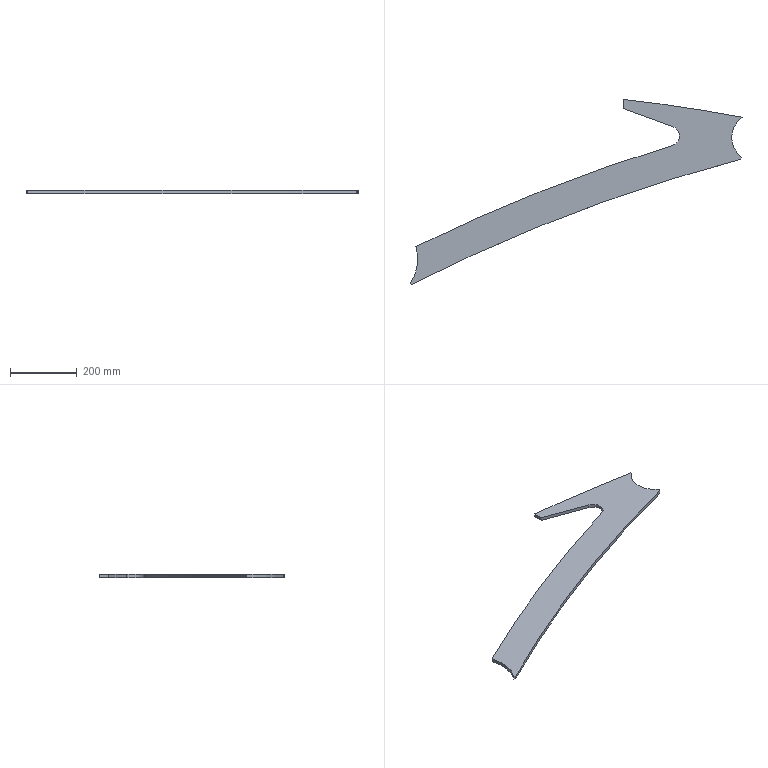Part | SolidWorks | features Extrusion 1 | 1 solid | 14 faces | box 997.777 x 556.587 x 10 mm | volume 1190658 mm3 | cylinder 7 | plane 7 | commonest cylinder face diameters 146 x2 60 x1 256 x1 9968 x1 10024 x1 10216 x1
STEP:
#1=CARTESIAN_POINT('',(1102.629,425.298,10.));
#2=VERTEX_POINT('',#1);
#3=CARTESIAN_POINT('',(1071.5,365.5,10.));
#4=VERTEX_POINT('',#3);
#5=CARTESIAN_POINT('',(1144.5,365.5,10.));
#6=DIRECTION('',(0.,0.,1.));
#7=DIRECTION('',(1.,0.,0.));
#8=AXIS2_PLACEMENT_3D('',#5,#6,#7);
#9=CIRCLE('',#8,73.);
#10=EDGE_CURVE('',#2,#4,#9,.T.);
#11=ORIENTED_EDGE('',*,*,#10,.T.);
#12=CARTESIAN_POINT('',(1071.5,365.5,0.));
#13=VERTEX_POINT('',#12);
#14=CARTESIAN_POINT('',(1071.5,365.5,10.));
#15=DIRECTION('',(0.,0.,-1.));
#16=VECTOR('',#15,1000.);
#17=LINE('',#14,#16);
#18=EDGE_CURVE('',#4,#13,#17,.T.);
#19=ORIENTED_EDGE('',*,*,#18,.T.);
#20=CARTESIAN_POINT('',(1102.629,425.298,0.));
#21=VERTEX_POINT('',#20);
#22=CARTESIAN_POINT('',(1144.5,365.5,0.));
#23=DIRECTION('',(0.,0.,1.));
#24=DIRECTION('',(1.,0.,0.));
#25=AXIS2_PLACEMENT_3D('',#22,#23,#24);
#26=CIRCLE('',#25,73.);
#27=EDGE_CURVE('',#21,#13,#26,.T.);
#28=ORIENTED_EDGE('',*,*,#27,.F.);
#29=CARTESIAN_POINT('',(1102.629,425.298,10.));
#30=DIRECTION('',(0.,0.,-1.));
#31=VECTOR('',#30,1000.);
#32=LINE('',#29,#31);
#33=EDGE_CURVE('',#2,#21,#32,.T.);
#34=ORIENTED_EDGE('',*,*,#33,.F.);
#35=EDGE_LOOP('',(#11,#19,#28,#34));
#36=FACE_OUTER_BOUND('',#35,.T.);
#37=CARTESIAN_POINT('',(1144.5,365.5,10.));
#38=DIRECTION('',(0.,0.,-1.));
#39=DIRECTION('',(-1.,0.,0.));
#40=AXIS2_PLACEMENT_3D('',#37,#38,#39);
#41=CYLINDRICAL_SURFACE('',#40,73.);
#42=ADVANCED_FACE('',(#36),#41,.F.);
#43=CARTESIAN_POINT('',(893.221,341.536,0.));
#44=VERTEX_POINT('',#43);
#45=CARTESIAN_POINT('',(894.771,398.434,0.));
#46=VERTEX_POINT('',#45);
#47=CARTESIAN_POINT('',(884.51,370.243,0.));
#48=DIRECTION('',(0.,0.,1.));
#49=DIRECTION('',(1.,0.,0.));
#50=AXIS2_PLACEMENT_3D('',#47,#48,#49);
#51=CIRCLE('',#50,30.);
#52=EDGE_CURVE('',#44,#46,#51,.T.);
#53=ORIENTED_EDGE('',*,*,#52,.F.);
#54=CARTESIAN_POINT('',(893.221,341.536,10.));
#55=VERTEX_POINT('',#54);
#56=CARTESIAN_POINT('',(893.221,341.536,10.));
#57=DIRECTION('',(0.,0.,-1.));
#58=VECTOR('',#57,1000.);
#59=LINE('',#56,#58);
#60=EDGE_CURVE('',#55,#44,#59,.T.);
#61=ORIENTED_EDGE('',*,*,#60,.F.);
#62=CARTESIAN_POINT('',(894.771,398.434,10.));
#63=VERTEX_POINT('',#62);
#64=CARTESIAN_POINT('',(884.51,370.243,10.));
#65=DIRECTION('',(0.,0.,1.));
#66=DIRECTION('',(1.,0.,0.));
#67=AXIS2_PLACEMENT_3D('',#64,#65,#66);
#68=CIRCLE('',#67,30.);
#69=EDGE_CURVE('',#55,#63,#68,.T.);
#70=ORIENTED_EDGE('',*,*,#69,.T.);
#71=CARTESIAN_POINT('',(894.771,398.434,10.));
#72=DIRECTION('',(0.,0.,-1.));
#73=VECTOR('',#72,1000.);
#74=LINE('',#71,#73);
#75=EDGE_CURVE('',#63,#46,#74,.T.);
#76=ORIENTED_EDGE('',*,*,#75,.T.);
#77=EDGE_LOOP('',(#53,#61,#70,#76));
#78=FACE_OUTER_BOUND('',#77,.T.);
#79=CARTESIAN_POINT('',(884.51,370.243,10.));
#80=DIRECTION('',(0.,0.,-1.));
#81=DIRECTION('',(-1.,0.,0.));
#82=AXIS2_PLACEMENT_3D('',#79,#80,#81);
#83=CYLINDRICAL_SURFACE('',#82,30.);
#84=ADVANCED_FACE('',(#78),#83,.F.);
#85=CARTESIAN_POINT('',(122.414,37.401,0.));
#86=VERTEX_POINT('',#85);
#87=CARTESIAN_POINT('',(2376.426,-4546.385,0.));
#88=DIRECTION('',(0.,0.,1.));
#89=DIRECTION('',(1.,0.,0.));
#90=AXIS2_PLACEMENT_3D('',#87,#88,#89);
#91=CIRCLE('',#90,5108.);
#92=EDGE_CURVE('',#44,#86,#91,.T.);
#93=ORIENTED_EDGE('',*,*,#92,.T.);
#94=CARTESIAN_POINT('',(122.414,37.401,10.));
#95=VERTEX_POINT('',#94);
#96=CARTESIAN_POINT('',(122.414,37.401,10.));
#97=DIRECTION('',(0.,0.,-1.));
#98=VECTOR('',#97,1000.);
#99=LINE('',#96,#98);
#100=EDGE_CURVE('',#95,#86,#99,.T.);
#101=ORIENTED_EDGE('',*,*,#100,.F.);
#102=CARTESIAN_POINT('',(2376.426,-4546.385,10.));
#103=DIRECTION('',(0.,0.,1.));
#104=DIRECTION('',(1.,0.,0.));
#105=AXIS2_PLACEMENT_3D('',#102,#103,#104);
#106=CIRCLE('',#105,5108.);
#107=EDGE_CURVE('',#55,#95,#106,.T.);
#108=ORIENTED_EDGE('',*,*,#107,.F.);
#109=ORIENTED_EDGE('',*,*,#60,.T.);
#110=EDGE_LOOP('',(#93,#101,#108,#109));
#111=FACE_OUTER_BOUND('',#110,.T.);
#112=CARTESIAN_POINT('',(2376.426,-4546.385,10.));
#113=DIRECTION('',(0.,0.,-1.));
#114=DIRECTION('',(-1.,0.,0.));
#115=AXIS2_PLACEMENT_3D('',#112,#113,#114);
#116=CYLINDRICAL_SURFACE('',#115,5108.);
#117=ADVANCED_FACE('',(#111),#116,.T.);
#118=CARTESIAN_POINT('',(104.851,-73.418,0.));
#119=VERTEX_POINT('',#118);
#120=CARTESIAN_POINT('',(0.,0.,0.));
#121=DIRECTION('',(0.,0.,1.));
#122=DIRECTION('',(1.,0.,0.));
#123=AXIS2_PLACEMENT_3D('',#120,#121,#122);
#124=CIRCLE('',#123,128.);
#125=EDGE_CURVE('',#119,#86,#124,.T.);
#126=ORIENTED_EDGE('',*,*,#125,.F.);
#127=CARTESIAN_POINT('',(104.851,-73.418,10.));
#128=VERTEX_POINT('',#127);
#129=CARTESIAN_POINT('',(104.851,-73.418,10.));
#130=DIRECTION('',(0.,0.,-1.));
#131=VECTOR('',#130,1000.);
#132=LINE('',#129,#131);
#133=EDGE_CURVE('',#128,#119,#132,.T.);
#134=ORIENTED_EDGE('',*,*,#133,.F.);
#135=CARTESIAN_POINT('',(0.,0.,10.));
#136=DIRECTION('',(0.,0.,1.));
#137=DIRECTION('',(1.,0.,0.));
#138=AXIS2_PLACEMENT_3D('',#135,#136,#137);
#139=CIRCLE('',#138,128.);
#140=EDGE_CURVE('',#128,#95,#139,.T.);
#141=ORIENTED_EDGE('',*,*,#140,.T.);
#142=ORIENTED_EDGE('',*,*,#100,.T.);
#143=EDGE_LOOP('',(#126,#134,#141,#142));
#144=FACE_OUTER_BOUND('',#143,.T.);
#145=CARTESIAN_POINT('',(0.,0.,10.));
#146=DIRECTION('',(0.,0.,-1.));
#147=DIRECTION('',(-1.,0.,0.));
#148=AXIS2_PLACEMENT_3D('',#145,#146,#147);
#149=CYLINDRICAL_SURFACE('',#148,128.);
#150=ADVANCED_FACE('',(#144),#149,.F.);
#151=CARTESIAN_POINT('',(109.235,-76.487,0.));
#152=VERTEX_POINT('',#151);
#153=CARTESIAN_POINT('',(782.756,-548.092,0.));
#154=DIRECTION('',(0.8192,-0.5736,0.));
#155=VECTOR('',#154,1000.);
#156=LINE('',#153,#155);
#157=EDGE_CURVE('',#119,#152,#156,.T.);
#158=ORIENTED_EDGE('',*,*,#157,.T.);
#159=CARTESIAN_POINT('',(109.235,-76.487,10.));
#160=VERTEX_POINT('',#159);
#161=CARTESIAN_POINT('',(109.235,-76.487,10.));
#162=DIRECTION('',(0.,0.,-1.));
#163=VECTOR('',#162,1000.);
#164=LINE('',#161,#163);
#165=EDGE_CURVE('',#160,#152,#164,.T.);
#166=ORIENTED_EDGE('',*,*,#165,.F.);
#167=CARTESIAN_POINT('',(782.756,-548.092,10.));
#168=DIRECTION('',(0.8192,-0.5736,0.));
#169=VECTOR('',#168,1000.);
#170=LINE('',#167,#169);
#171=EDGE_CURVE('',#128,#160,#170,.T.);
#172=ORIENTED_EDGE('',*,*,#171,.F.);
#173=ORIENTED_EDGE('',*,*,#133,.T.);
#174=EDGE_LOOP('',(#158,#166,#172,#173));
#175=FACE_OUTER_BOUND('',#174,.T.);
#176=CARTESIAN_POINT('',(782.756,-548.092,10.));
#177=DIRECTION('',(0.5736,0.8192,0.));
#178=DIRECTION('',(-0.8192,0.5736,0.));
#179=AXIS2_PLACEMENT_3D('',#176,#177,#178);
#180=PLANE('',#179);
#181=ADVANCED_FACE('',(#175),#180,.F.);
#182=CARTESIAN_POINT('',(1098.632,299.994,0.));
#183=VERTEX_POINT('',#182);
#184=CARTESIAN_POINT('',(2376.426,-4546.385,0.));
#185=DIRECTION('',(0.,0.,1.));
#186=DIRECTION('',(1.,0.,0.));
#187=AXIS2_PLACEMENT_3D('',#184,#185,#186);
#188=CIRCLE('',#187,5012.);
#189=EDGE_CURVE('',#183,#152,#188,.T.);
#190=ORIENTED_EDGE('',*,*,#189,.F.);
#191=CARTESIAN_POINT('',(1098.632,299.994,10.));
#192=VERTEX_POINT('',#191);
#193=CARTESIAN_POINT('',(1098.632,299.994,10.));
#194=DIRECTION('',(0.,0.,-1.));
#195=VECTOR('',#194,1000.);
#196=LINE('',#193,#195);
#197=EDGE_CURVE('',#192,#183,#196,.T.);
#198=ORIENTED_EDGE('',*,*,#197,.F.);
#199=CARTESIAN_POINT('',(2376.426,-4546.385,10.));
#200=DIRECTION('',(0.,0.,1.));
#201=DIRECTION('',(1.,0.,0.));
#202=AXIS2_PLACEMENT_3D('',#199,#200,#201);
#203=CIRCLE('',#202,5012.);
#204=EDGE_CURVE('',#192,#160,#203,.T.);
#205=ORIENTED_EDGE('',*,*,#204,.T.);
#206=ORIENTED_EDGE('',*,*,#165,.T.);
#207=EDGE_LOOP('',(#190,#198,#205,#206));
#208=FACE_OUTER_BOUND('',#207,.T.);
#209=CARTESIAN_POINT('',(2376.426,-4546.385,10.));
#210=DIRECTION('',(0.,0.,-1.));
#211=DIRECTION('',(-1.,0.,0.));
#212=AXIS2_PLACEMENT_3D('',#209,#210,#211);
#213=CYLINDRICAL_SURFACE('',#212,5012.);
#214=ADVANCED_FACE('',(#208),#213,.F.);
#215=CARTESIAN_POINT('',(1102.629,305.702,0.));
#216=VERTEX_POINT('',#215);
#217=CARTESIAN_POINT('',(440.255,-640.266,0.));
#218=DIRECTION('',(-0.5736,-0.8192,0.));
#219=VECTOR('',#218,1000.);
#220=LINE('',#217,#219);
#221=EDGE_CURVE('',#216,#183,#220,.T.);
#222=ORIENTED_EDGE('',*,*,#221,.F.);
#223=CARTESIAN_POINT('',(1102.629,305.702,10.));
#224=VERTEX_POINT('',#223);
#225=CARTESIAN_POINT('',(1102.629,305.702,10.));
#226=DIRECTION('',(0.,0.,-1.));
#227=VECTOR('',#226,1000.);
#228=LINE('',#225,#227);
#229=EDGE_CURVE('',#224,#216,#228,.T.);
#230=ORIENTED_EDGE('',*,*,#229,.F.);
#231=CARTESIAN_POINT('',(440.255,-640.266,10.));
#232=DIRECTION('',(-0.5736,-0.8192,0.));
#233=VECTOR('',#232,1000.);
#234=LINE('',#231,#233);
#235=EDGE_CURVE('',#224,#192,#234,.T.);
#236=ORIENTED_EDGE('',*,*,#235,.T.);
#237=ORIENTED_EDGE('',*,*,#197,.T.);
#238=EDGE_LOOP('',(#222,#230,#236,#237));
#239=FACE_OUTER_BOUND('',#238,.T.);
#240=CARTESIAN_POINT('',(440.255,-640.266,10.));
#241=DIRECTION('',(0.8192,-0.5736,0.));
#242=DIRECTION('',(0.5736,0.8192,0.));
#243=AXIS2_PLACEMENT_3D('',#240,#241,#242);
#244=PLANE('',#243);
#245=ADVANCED_FACE('',(#239),#244,.T.);
#246=ORIENTED_EDGE('',*,*,#18,.F.);
#247=CARTESIAN_POINT('',(1144.5,365.5,10.));
#248=DIRECTION('',(0.,0.,1.));
#249=DIRECTION('',(1.,0.,0.));
#250=AXIS2_PLACEMENT_3D('',#247,#248,#249);
#251=CIRCLE('',#250,73.);
#252=EDGE_CURVE('',#4,#224,#251,.T.);
#253=ORIENTED_EDGE('',*,*,#252,.T.);
#254=ORIENTED_EDGE('',*,*,#229,.T.);
#255=CARTESIAN_POINT('',(1144.5,365.5,0.));
#256=DIRECTION('',(0.,0.,1.));
#257=DIRECTION('',(1.,0.,0.));
#258=AXIS2_PLACEMENT_3D('',#255,#256,#257);
#259=CIRCLE('',#258,73.);
#260=EDGE_CURVE('',#13,#216,#259,.T.);
#261=ORIENTED_EDGE('',*,*,#260,.F.);
#262=EDGE_LOOP('',(#246,#253,#254,#261));
#263=FACE_OUTER_BOUND('',#262,.T.);
#264=CARTESIAN_POINT('',(1144.5,365.5,10.));
#265=DIRECTION('',(0.,0.,-1.));
#266=DIRECTION('',(-1.,0.,0.));
#267=AXIS2_PLACEMENT_3D('',#264,#265,#266);
#268=CYLINDRICAL_SURFACE('',#267,73.);
#269=ADVANCED_FACE('',(#263),#268,.F.);
#270=CARTESIAN_POINT('',(1101.599,426.768,0.));
#271=VERTEX_POINT('',#270);
#272=CARTESIAN_POINT('',(1508.088,-153.758,0.));
#273=DIRECTION('',(-0.5736,0.8192,0.));
#274=VECTOR('',#273,1000.);
#275=LINE('',#272,#274);
#276=EDGE_CURVE('',#21,#271,#275,.T.);
#277=ORIENTED_EDGE('',*,*,#276,.T.);
#278=CARTESIAN_POINT('',(1101.599,426.768,10.));
#279=VERTEX_POINT('',#278);
#280=CARTESIAN_POINT('',(1101.599,426.768,10.));
#281=DIRECTION('',(0.,0.,-1.));
#282=VECTOR('',#281,1000.);
#283=LINE('',#280,#282);
#284=EDGE_CURVE('',#279,#271,#283,.T.);
#285=ORIENTED_EDGE('',*,*,#284,.F.);
#286=CARTESIAN_POINT('',(1508.088,-153.758,10.));
#287=DIRECTION('',(-0.5736,0.8192,0.));
#288=VECTOR('',#287,1000.);
#289=LINE('',#286,#288);
#290=EDGE_CURVE('',#2,#279,#289,.T.);
#291=ORIENTED_EDGE('',*,*,#290,.F.);
#292=ORIENTED_EDGE('',*,*,#33,.T.);
#293=EDGE_LOOP('',(#277,#285,#291,#292));
#294=FACE_OUTER_BOUND('',#293,.T.);
#295=CARTESIAN_POINT('',(1508.088,-153.758,10.));
#296=DIRECTION('',(-0.8192,-0.5736,0.));
#297=DIRECTION('',(0.5736,-0.8192,0.));
#298=AXIS2_PLACEMENT_3D('',#295,#296,#297);
#299=PLANE('',#298);
#300=ADVANCED_FACE('',(#294),#299,.F.);
#301=CARTESIAN_POINT('',(746.5,480.1,0.));
#302=VERTEX_POINT('',#301);
#303=CARTESIAN_POINT('',(184.296,-4472.09,0.));
#304=DIRECTION('',(0.,0.,1.));
#305=DIRECTION('',(1.,0.,0.));
#306=AXIS2_PLACEMENT_3D('',#303,#304,#305);
#307=CIRCLE('',#306,4984.);
#308=EDGE_CURVE('',#271,#302,#307,.T.);
#309=ORIENTED_EDGE('',*,*,#308,.T.);
#310=CARTESIAN_POINT('',(746.5,480.1,10.));
#311=VERTEX_POINT('',#310);
#312=CARTESIAN_POINT('',(746.5,480.1,10.));
#313=DIRECTION('',(0.,0.,-1.));
#314=VECTOR('',#313,1000.);
#315=LINE('',#312,#314);
#316=EDGE_CURVE('',#311,#302,#315,.T.);
#317=ORIENTED_EDGE('',*,*,#316,.F.);
#318=CARTESIAN_POINT('',(184.296,-4472.09,10.));
#319=DIRECTION('',(0.,0.,1.));
#320=DIRECTION('',(1.,0.,0.));
#321=AXIS2_PLACEMENT_3D('',#318,#319,#320);
#322=CIRCLE('',#321,4984.);
#323=EDGE_CURVE('',#279,#311,#322,.T.);
#324=ORIENTED_EDGE('',*,*,#323,.F.);
#325=ORIENTED_EDGE('',*,*,#284,.T.);
#326=EDGE_LOOP('',(#309,#317,#324,#325));
#327=FACE_OUTER_BOUND('',#326,.T.);
#328=CARTESIAN_POINT('',(184.296,-4472.09,10.));
#329=DIRECTION('',(0.,0.,-1.));
#330=DIRECTION('',(-1.,0.,0.));
#331=AXIS2_PLACEMENT_3D('',#328,#329,#330);
#332=CYLINDRICAL_SURFACE('',#331,4984.);
#333=ADVANCED_FACE('',(#327),#332,.T.);
#334=CARTESIAN_POINT('',(746.5,452.4,0.));
#335=VERTEX_POINT('',#334);
#336=CARTESIAN_POINT('',(746.5,-770.864,0.));
#337=DIRECTION('',(0.,-1.,0.));
#338=VECTOR('',#337,1000.);
#339=LINE('',#336,#338);
#340=EDGE_CURVE('',#302,#335,#339,.T.);
#341=ORIENTED_EDGE('',*,*,#340,.T.);
#342=CARTESIAN_POINT('',(746.5,452.4,10.));
#343=VERTEX_POINT('',#342);
#344=CARTESIAN_POINT('',(746.5,452.4,10.));
#345=DIRECTION('',(0.,0.,-1.));
#346=VECTOR('',#345,1000.);
#347=LINE('',#344,#346);
#348=EDGE_CURVE('',#343,#335,#347,.T.);
#349=ORIENTED_EDGE('',*,*,#348,.F.);
#350=CARTESIAN_POINT('',(746.5,-770.864,10.));
#351=DIRECTION('',(0.,-1.,0.));
#352=VECTOR('',#351,1000.);
#353=LINE('',#350,#352);
#354=EDGE_CURVE('',#311,#343,#353,.T.);
#355=ORIENTED_EDGE('',*,*,#354,.F.);
#356=ORIENTED_EDGE('',*,*,#316,.T.);
#357=EDGE_LOOP('',(#341,#349,#355,#356));
#358=FACE_OUTER_BOUND('',#357,.T.);
#359=CARTESIAN_POINT('',(746.5,-770.864,10.));
#360=DIRECTION('',(1.,0.,0.));
#361=DIRECTION('',(0.,0.,-1.));
#362=AXIS2_PLACEMENT_3D('',#359,#360,#361);
#363=PLANE('',#362);
#364=ADVANCED_FACE('',(#358),#363,.F.);
#365=CARTESIAN_POINT('',(1033.925,347.786,0.));
#366=DIRECTION('',(0.9397,-0.342,0.));
#367=VECTOR('',#366,1000.);
#368=LINE('',#365,#367);
#369=EDGE_CURVE('',#335,#46,#368,.T.);
#370=ORIENTED_EDGE('',*,*,#369,.T.);
#371=ORIENTED_EDGE('',*,*,#75,.F.);
#372=CARTESIAN_POINT('',(1033.925,347.786,10.));
#373=DIRECTION('',(0.9397,-0.342,0.));
#374=VECTOR('',#373,1000.);
#375=LINE('',#372,#374);
#376=EDGE_CURVE('',#343,#63,#375,.T.);
#377=ORIENTED_EDGE('',*,*,#376,.F.);
#378=ORIENTED_EDGE('',*,*,#348,.T.);
#379=EDGE_LOOP('',(#370,#371,#377,#378));
#380=FACE_OUTER_BOUND('',#379,.T.);
#381=CARTESIAN_POINT('',(1033.925,347.786,10.));
#382=DIRECTION('',(0.342,0.9397,0.));
#383=DIRECTION('',(-0.9397,0.342,0.));
#384=AXIS2_PLACEMENT_3D('',#381,#382,#383);
#385=PLANE('',#384);
#386=ADVANCED_FACE('',(#380),#385,.F.);
#387=ORIENTED_EDGE('',*,*,#69,.F.);
#388=ORIENTED_EDGE('',*,*,#107,.T.);
#389=ORIENTED_EDGE('',*,*,#140,.F.);
#390=ORIENTED_EDGE('',*,*,#171,.T.);
#391=ORIENTED_EDGE('',*,*,#204,.F.);
#392=ORIENTED_EDGE('',*,*,#235,.F.);
#393=ORIENTED_EDGE('',*,*,#252,.F.);
#394=ORIENTED_EDGE('',*,*,#10,.F.);
#395=ORIENTED_EDGE('',*,*,#290,.T.);
#396=ORIENTED_EDGE('',*,*,#323,.T.);
#397=ORIENTED_EDGE('',*,*,#354,.T.);
#398=ORIENTED_EDGE('',*,*,#376,.T.);
#399=EDGE_LOOP('',(#387,#388,#389,#390,#391,#392,#393,#394,#395,#396,#397,#398));
#400=FACE_OUTER_BOUND('',#399,.T.);
#401=CARTESIAN_POINT('',(626.769,-770.864,10.));
#402=DIRECTION('',(0.,0.,1.));
#403=DIRECTION('',(1.,0.,0.));
#404=AXIS2_PLACEMENT_3D('',#401,#402,#403);
#405=PLANE('',#404);
#406=ADVANCED_FACE('',(#400),#405,.T.);
#407=ORIENTED_EDGE('',*,*,#52,.T.);
#408=ORIENTED_EDGE('',*,*,#369,.F.);
#409=ORIENTED_EDGE('',*,*,#340,.F.);
#410=ORIENTED_EDGE('',*,*,#308,.F.);
#411=ORIENTED_EDGE('',*,*,#276,.F.);
#412=ORIENTED_EDGE('',*,*,#27,.T.);
#413=ORIENTED_EDGE('',*,*,#260,.T.);
#414=ORIENTED_EDGE('',*,*,#221,.T.);
#415=ORIENTED_EDGE('',*,*,#189,.T.);
#416=ORIENTED_EDGE('',*,*,#157,.F.);
#417=ORIENTED_EDGE('',*,*,#125,.T.);
#418=ORIENTED_EDGE('',*,*,#92,.F.);
#419=EDGE_LOOP('',(#407,#408,#409,#410,#411,#412,#413,#414,#415,#416,#417,#418));
#420=FACE_OUTER_BOUND('',#419,.T.);
#421=CARTESIAN_POINT('',(626.769,-770.864,0.));
#422=DIRECTION('',(0.,0.,1.));
#423=DIRECTION('',(1.,0.,0.));
#424=AXIS2_PLACEMENT_3D('',#421,#422,#423);
#425=PLANE('',#424);
#426=ADVANCED_FACE('',(#420),#425,.F.);
#427=CLOSED_SHELL('',(#42,#84,#117,#150,#181,#214,#245,#269,#300,#333,#364,#386,#406,#426));
#428=MANIFOLD_SOLID_BREP('',#427);
#429=CARTESIAN_POINT('',(0.,0.,0.));
#430=DIRECTION('',(0.,0.,1.));
#431=DIRECTION('',(1.,0.,0.));
#432=AXIS2_PLACEMENT_3D('',#429,#430,#431);
#433=(LENGTH_UNIT()NAMED_UNIT(*)SI_UNIT(.MILLI.,.METRE.));
#434=UNCERTAINTY_MEASURE_WITH_UNIT(LENGTH_MEASURE(0.00001),#433,'','');
#435=(NAMED_UNIT(*)PLANE_ANGLE_UNIT()SI_UNIT($,.RADIAN.));
#436=(NAMED_UNIT(*)SI_UNIT($,.STERADIAN.)SOLID_ANGLE_UNIT());
#437=(GEOMETRIC_REPRESENTATION_CONTEXT(3)GLOBAL_UNCERTAINTY_ASSIGNED_CONTEXT((#434))GLOBAL_UNIT_ASSIGNED_CONTEXT((#433,#435,#436))REPRESENTATION_CONTEXT('',''));
#438=ADVANCED_BREP_SHAPE_REPRESENTATION('',(#428,#432),#437);